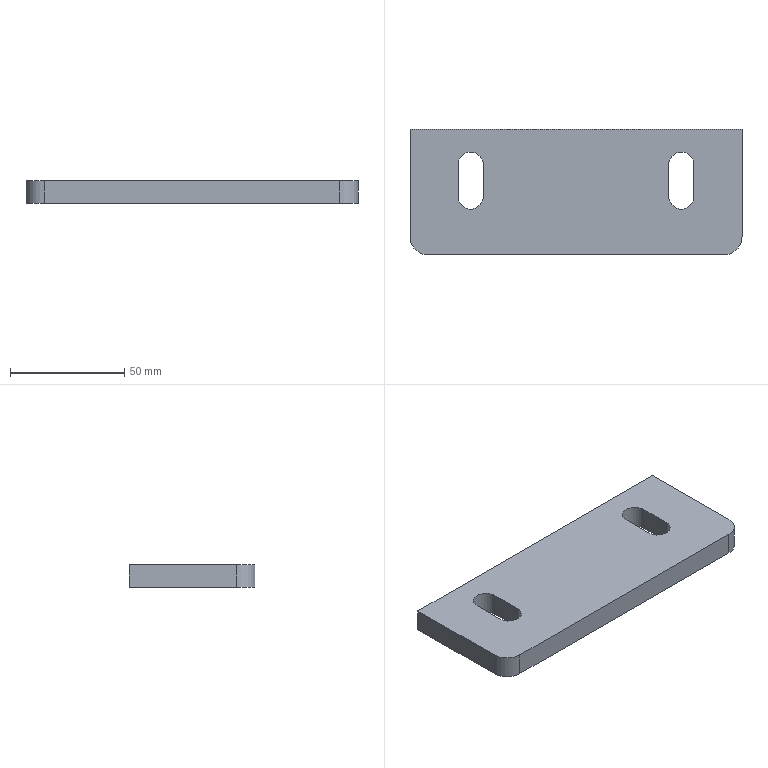Part | SolidWorks | features Extrusion 1, Fillet 1, ICE 1 | 1 solid | 16 faces | box 145 x 55 x 10 mm | volume 74495 mm3 | plane 10 | cylinder 6 | commonest cylinder face diameters 11 x4 16 x2
STEP:
#1=CARTESIAN_POINT('',(-72.5,27.5,0.));
#2=VERTEX_POINT('',#1);
#3=CARTESIAN_POINT('',(-72.5,-19.5,0.));
#4=VERTEX_POINT('',#3);
#5=CARTESIAN_POINT('',(-72.5,27.5,0.));
#6=DIRECTION('',(0.,-1.,0.));
#7=VECTOR('',#6,1000.);
#8=LINE('',#5,#7);
#9=EDGE_CURVE('',#2,#4,#8,.T.);
#10=ORIENTED_EDGE('',*,*,#9,.T.);
#11=CARTESIAN_POINT('',(-72.5,-19.5,10.));
#12=VERTEX_POINT('',#11);
#13=CARTESIAN_POINT('',(-72.5,-19.5,10.));
#14=DIRECTION('',(0.,0.,1.));
#15=VECTOR('',#14,1000.);
#16=LINE('',#13,#15);
#17=EDGE_CURVE('',#4,#12,#16,.T.);
#18=ORIENTED_EDGE('',*,*,#17,.T.);
#19=CARTESIAN_POINT('',(-72.5,27.5,10.));
#20=VERTEX_POINT('',#19);
#21=CARTESIAN_POINT('',(-72.5,27.5,10.));
#22=DIRECTION('',(0.,-1.,0.));
#23=VECTOR('',#22,1000.);
#24=LINE('',#21,#23);
#25=EDGE_CURVE('',#20,#12,#24,.T.);
#26=ORIENTED_EDGE('',*,*,#25,.F.);
#27=CARTESIAN_POINT('',(-72.5,27.5,10.));
#28=DIRECTION('',(0.,0.,-1.));
#29=VECTOR('',#28,1000.);
#30=LINE('',#27,#29);
#31=EDGE_CURVE('',#20,#2,#30,.T.);
#32=ORIENTED_EDGE('',*,*,#31,.T.);
#33=EDGE_LOOP('',(#10,#18,#26,#32));
#34=FACE_OUTER_BOUND('',#33,.T.);
#35=CARTESIAN_POINT('',(-72.5,27.5,10.));
#36=DIRECTION('',(1.,0.,0.));
#37=DIRECTION('',(0.,1.,0.));
#38=AXIS2_PLACEMENT_3D('',#35,#36,#37);
#39=PLANE('',#38);
#40=ADVANCED_FACE('',(#34),#39,.F.);
#41=CARTESIAN_POINT('',(-64.5,-27.5,0.));
#42=VERTEX_POINT('',#41);
#43=CARTESIAN_POINT('',(64.5,-27.5,0.));
#44=VERTEX_POINT('',#43);
#45=CARTESIAN_POINT('',(72.5,-27.5,0.));
#46=DIRECTION('',(1.,0.,0.));
#47=VECTOR('',#46,1000.);
#48=LINE('',#45,#47);
#49=EDGE_CURVE('',#42,#44,#48,.T.);
#50=ORIENTED_EDGE('',*,*,#49,.T.);
#51=CARTESIAN_POINT('',(64.5,-27.5,10.));
#52=VERTEX_POINT('',#51);
#53=CARTESIAN_POINT('',(64.5,-27.5,10.));
#54=DIRECTION('',(0.,0.,1.));
#55=VECTOR('',#54,1000.);
#56=LINE('',#53,#55);
#57=EDGE_CURVE('',#44,#52,#56,.T.);
#58=ORIENTED_EDGE('',*,*,#57,.T.);
#59=CARTESIAN_POINT('',(-64.5,-27.5,10.));
#60=VERTEX_POINT('',#59);
#61=CARTESIAN_POINT('',(72.5,-27.5,10.));
#62=DIRECTION('',(1.,0.,0.));
#63=VECTOR('',#62,1000.);
#64=LINE('',#61,#63);
#65=EDGE_CURVE('',#60,#52,#64,.T.);
#66=ORIENTED_EDGE('',*,*,#65,.F.);
#67=CARTESIAN_POINT('',(-64.5,-27.5,10.));
#68=DIRECTION('',(0.,0.,-1.));
#69=VECTOR('',#68,1000.);
#70=LINE('',#67,#69);
#71=EDGE_CURVE('',#60,#42,#70,.T.);
#72=ORIENTED_EDGE('',*,*,#71,.T.);
#73=EDGE_LOOP('',(#50,#58,#66,#72));
#74=FACE_OUTER_BOUND('',#73,.T.);
#75=CARTESIAN_POINT('',(72.5,-27.5,10.));
#76=DIRECTION('',(0.,1.,0.));
#77=DIRECTION('',(-1.,0.,0.));
#78=AXIS2_PLACEMENT_3D('',#75,#76,#77);
#79=PLANE('',#78);
#80=ADVANCED_FACE('',(#74),#79,.F.);
#81=CARTESIAN_POINT('',(72.5,-19.5,10.));
#82=VERTEX_POINT('',#81);
#83=CARTESIAN_POINT('',(72.5,27.5,10.));
#84=VERTEX_POINT('',#83);
#85=CARTESIAN_POINT('',(72.5,27.5,10.));
#86=DIRECTION('',(0.,1.,0.));
#87=VECTOR('',#86,1000.);
#88=LINE('',#85,#87);
#89=EDGE_CURVE('',#82,#84,#88,.T.);
#90=ORIENTED_EDGE('',*,*,#89,.F.);
#91=CARTESIAN_POINT('',(72.5,-19.5,0.));
#92=VERTEX_POINT('',#91);
#93=CARTESIAN_POINT('',(72.5,-19.5,10.));
#94=DIRECTION('',(0.,0.,-1.));
#95=VECTOR('',#94,1000.);
#96=LINE('',#93,#95);
#97=EDGE_CURVE('',#82,#92,#96,.T.);
#98=ORIENTED_EDGE('',*,*,#97,.T.);
#99=CARTESIAN_POINT('',(72.5,27.5,0.));
#100=VERTEX_POINT('',#99);
#101=CARTESIAN_POINT('',(72.5,27.5,0.));
#102=DIRECTION('',(0.,1.,0.));
#103=VECTOR('',#102,1000.);
#104=LINE('',#101,#103);
#105=EDGE_CURVE('',#92,#100,#104,.T.);
#106=ORIENTED_EDGE('',*,*,#105,.T.);
#107=CARTESIAN_POINT('',(72.5,27.5,10.));
#108=DIRECTION('',(0.,0.,-1.));
#109=VECTOR('',#108,1000.);
#110=LINE('',#107,#109);
#111=EDGE_CURVE('',#84,#100,#110,.T.);
#112=ORIENTED_EDGE('',*,*,#111,.F.);
#113=EDGE_LOOP('',(#90,#98,#106,#112));
#114=FACE_OUTER_BOUND('',#113,.T.);
#115=CARTESIAN_POINT('',(72.5,27.5,10.));
#116=DIRECTION('',(-1.,0.,0.));
#117=DIRECTION('',(0.,0.,1.));
#118=AXIS2_PLACEMENT_3D('',#115,#116,#117);
#119=PLANE('',#118);
#120=ADVANCED_FACE('',(#114),#119,.F.);
#121=CARTESIAN_POINT('',(72.5,27.5,0.));
#122=DIRECTION('',(-1.,0.,0.));
#123=VECTOR('',#122,1000.);
#124=LINE('',#121,#123);
#125=EDGE_CURVE('',#100,#2,#124,.T.);
#126=ORIENTED_EDGE('',*,*,#125,.T.);
#127=ORIENTED_EDGE('',*,*,#31,.F.);
#128=CARTESIAN_POINT('',(72.5,27.5,10.));
#129=DIRECTION('',(-1.,0.,0.));
#130=VECTOR('',#129,1000.);
#131=LINE('',#128,#130);
#132=EDGE_CURVE('',#84,#20,#131,.T.);
#133=ORIENTED_EDGE('',*,*,#132,.F.);
#134=ORIENTED_EDGE('',*,*,#111,.T.);
#135=EDGE_LOOP('',(#126,#127,#133,#134));
#136=FACE_OUTER_BOUND('',#135,.T.);
#137=CARTESIAN_POINT('',(72.5,27.5,10.));
#138=DIRECTION('',(0.,-1.,0.));
#139=DIRECTION('',(1.,0.,0.));
#140=AXIS2_PLACEMENT_3D('',#137,#138,#139);
#141=PLANE('',#140);
#142=ADVANCED_FACE('',(#136),#141,.F.);
#143=CARTESIAN_POINT('',(40.5,12.,10.));
#144=VERTEX_POINT('',#143);
#145=CARTESIAN_POINT('',(40.5,-2.,10.));
#146=VERTEX_POINT('',#145);
#147=CARTESIAN_POINT('',(40.5,12.,10.));
#148=DIRECTION('',(0.,-1.,0.));
#149=VECTOR('',#148,1000.);
#150=LINE('',#147,#149);
#151=EDGE_CURVE('',#144,#146,#150,.T.);
#152=ORIENTED_EDGE('',*,*,#151,.F.);
#153=CARTESIAN_POINT('',(51.5,12.,10.));
#154=VERTEX_POINT('',#153);
#155=CARTESIAN_POINT('',(46.,12.,10.));
#156=DIRECTION('',(0.,0.,1.));
#157=DIRECTION('',(1.,0.,0.));
#158=AXIS2_PLACEMENT_3D('',#155,#156,#157);
#159=CIRCLE('',#158,5.5);
#160=EDGE_CURVE('',#154,#144,#159,.T.);
#161=ORIENTED_EDGE('',*,*,#160,.F.);
#162=CARTESIAN_POINT('',(51.5,-2.,10.));
#163=VERTEX_POINT('',#162);
#164=CARTESIAN_POINT('',(51.5,12.,10.));
#165=DIRECTION('',(0.,1.,0.));
#166=VECTOR('',#165,1000.);
#167=LINE('',#164,#166);
#168=EDGE_CURVE('',#163,#154,#167,.T.);
#169=ORIENTED_EDGE('',*,*,#168,.F.);
#170=CARTESIAN_POINT('',(46.,-2.,10.));
#171=DIRECTION('',(0.,0.,1.));
#172=DIRECTION('',(1.,0.,0.));
#173=AXIS2_PLACEMENT_3D('',#170,#171,#172);
#174=CIRCLE('',#173,5.5);
#175=EDGE_CURVE('',#146,#163,#174,.T.);
#176=ORIENTED_EDGE('',*,*,#175,.F.);
#177=EDGE_LOOP('',(#152,#161,#169,#176));
#178=FACE_BOUND('',#177,.T.);
#179=CARTESIAN_POINT('',(-51.5,12.,10.));
#180=VERTEX_POINT('',#179);
#181=CARTESIAN_POINT('',(-51.5,-2.,10.));
#182=VERTEX_POINT('',#181);
#183=CARTESIAN_POINT('',(-51.5,12.,10.));
#184=DIRECTION('',(0.,-1.,0.));
#185=VECTOR('',#184,1000.);
#186=LINE('',#183,#185);
#187=EDGE_CURVE('',#180,#182,#186,.T.);
#188=ORIENTED_EDGE('',*,*,#187,.F.);
#189=CARTESIAN_POINT('',(-40.5,12.,10.));
#190=VERTEX_POINT('',#189);
#191=CARTESIAN_POINT('',(-46.,12.,10.));
#192=DIRECTION('',(0.,0.,1.));
#193=DIRECTION('',(1.,0.,0.));
#194=AXIS2_PLACEMENT_3D('',#191,#192,#193);
#195=CIRCLE('',#194,5.5);
#196=EDGE_CURVE('',#190,#180,#195,.T.);
#197=ORIENTED_EDGE('',*,*,#196,.F.);
#198=CARTESIAN_POINT('',(-40.5,-2.,10.));
#199=VERTEX_POINT('',#198);
#200=CARTESIAN_POINT('',(-40.5,12.,10.));
#201=DIRECTION('',(0.,1.,0.));
#202=VECTOR('',#201,1000.);
#203=LINE('',#200,#202);
#204=EDGE_CURVE('',#199,#190,#203,.T.);
#205=ORIENTED_EDGE('',*,*,#204,.F.);
#206=CARTESIAN_POINT('',(-46.,-2.,10.));
#207=DIRECTION('',(0.,0.,1.));
#208=DIRECTION('',(1.,0.,0.));
#209=AXIS2_PLACEMENT_3D('',#206,#207,#208);
#210=CIRCLE('',#209,5.5);
#211=EDGE_CURVE('',#182,#199,#210,.T.);
#212=ORIENTED_EDGE('',*,*,#211,.F.);
#213=EDGE_LOOP('',(#188,#197,#205,#212));
#214=FACE_BOUND('',#213,.T.);
#215=ORIENTED_EDGE('',*,*,#65,.T.);
#216=CARTESIAN_POINT('',(64.5,-19.5,10.));
#217=DIRECTION('',(0.,0.,1.));
#218=DIRECTION('',(-1.,0.,0.));
#219=AXIS2_PLACEMENT_3D('',#216,#217,#218);
#220=CIRCLE('',#219,8.);
#221=EDGE_CURVE('',#52,#82,#220,.T.);
#222=ORIENTED_EDGE('',*,*,#221,.T.);
#223=ORIENTED_EDGE('',*,*,#89,.T.);
#224=ORIENTED_EDGE('',*,*,#132,.T.);
#225=ORIENTED_EDGE('',*,*,#25,.T.);
#226=CARTESIAN_POINT('',(-64.5,-19.5,10.));
#227=DIRECTION('',(0.,0.,1.));
#228=DIRECTION('',(-1.,0.,0.));
#229=AXIS2_PLACEMENT_3D('',#226,#227,#228);
#230=CIRCLE('',#229,8.);
#231=EDGE_CURVE('',#12,#60,#230,.T.);
#232=ORIENTED_EDGE('',*,*,#231,.T.);
#233=EDGE_LOOP('',(#215,#222,#223,#224,#225,#232));
#234=FACE_OUTER_BOUND('',#233,.T.);
#235=CARTESIAN_POINT('',(0.,0.,10.));
#236=DIRECTION('',(0.,0.,-1.));
#237=DIRECTION('',(-1.,0.,0.));
#238=AXIS2_PLACEMENT_3D('',#235,#236,#237);
#239=PLANE('',#238);
#240=ADVANCED_FACE('',(#178,#214,#234),#239,.F.);
#241=CARTESIAN_POINT('',(51.5,12.,0.));
#242=VERTEX_POINT('',#241);
#243=CARTESIAN_POINT('',(40.5,12.,0.));
#244=VERTEX_POINT('',#243);
#245=CARTESIAN_POINT('',(46.,12.,0.));
#246=DIRECTION('',(0.,0.,1.));
#247=DIRECTION('',(1.,0.,0.));
#248=AXIS2_PLACEMENT_3D('',#245,#246,#247);
#249=CIRCLE('',#248,5.5);
#250=EDGE_CURVE('',#242,#244,#249,.T.);
#251=ORIENTED_EDGE('',*,*,#250,.T.);
#252=CARTESIAN_POINT('',(40.5,-2.,0.));
#253=VERTEX_POINT('',#252);
#254=CARTESIAN_POINT('',(40.5,12.,0.));
#255=DIRECTION('',(0.,-1.,0.));
#256=VECTOR('',#255,1000.);
#257=LINE('',#254,#256);
#258=EDGE_CURVE('',#244,#253,#257,.T.);
#259=ORIENTED_EDGE('',*,*,#258,.T.);
#260=CARTESIAN_POINT('',(51.5,-2.,0.));
#261=VERTEX_POINT('',#260);
#262=CARTESIAN_POINT('',(46.,-2.,0.));
#263=DIRECTION('',(0.,0.,1.));
#264=DIRECTION('',(1.,0.,0.));
#265=AXIS2_PLACEMENT_3D('',#262,#263,#264);
#266=CIRCLE('',#265,5.5);
#267=EDGE_CURVE('',#253,#261,#266,.T.);
#268=ORIENTED_EDGE('',*,*,#267,.T.);
#269=CARTESIAN_POINT('',(51.5,12.,0.));
#270=DIRECTION('',(0.,1.,0.));
#271=VECTOR('',#270,1000.);
#272=LINE('',#269,#271);
#273=EDGE_CURVE('',#261,#242,#272,.T.);
#274=ORIENTED_EDGE('',*,*,#273,.T.);
#275=EDGE_LOOP('',(#251,#259,#268,#274));
#276=FACE_BOUND('',#275,.T.);
#277=CARTESIAN_POINT('',(-40.5,12.,0.));
#278=VERTEX_POINT('',#277);
#279=CARTESIAN_POINT('',(-51.5,12.,0.));
#280=VERTEX_POINT('',#279);
#281=CARTESIAN_POINT('',(-46.,12.,0.));
#282=DIRECTION('',(0.,0.,1.));
#283=DIRECTION('',(1.,0.,0.));
#284=AXIS2_PLACEMENT_3D('',#281,#282,#283);
#285=CIRCLE('',#284,5.5);
#286=EDGE_CURVE('',#278,#280,#285,.T.);
#287=ORIENTED_EDGE('',*,*,#286,.T.);
#288=CARTESIAN_POINT('',(-51.5,-2.,0.));
#289=VERTEX_POINT('',#288);
#290=CARTESIAN_POINT('',(-51.5,12.,0.));
#291=DIRECTION('',(0.,-1.,0.));
#292=VECTOR('',#291,1000.);
#293=LINE('',#290,#292);
#294=EDGE_CURVE('',#280,#289,#293,.T.);
#295=ORIENTED_EDGE('',*,*,#294,.T.);
#296=CARTESIAN_POINT('',(-40.5,-2.,0.));
#297=VERTEX_POINT('',#296);
#298=CARTESIAN_POINT('',(-46.,-2.,0.));
#299=DIRECTION('',(0.,0.,1.));
#300=DIRECTION('',(1.,0.,0.));
#301=AXIS2_PLACEMENT_3D('',#298,#299,#300);
#302=CIRCLE('',#301,5.5);
#303=EDGE_CURVE('',#289,#297,#302,.T.);
#304=ORIENTED_EDGE('',*,*,#303,.T.);
#305=CARTESIAN_POINT('',(-40.5,12.,0.));
#306=DIRECTION('',(0.,1.,0.));
#307=VECTOR('',#306,1000.);
#308=LINE('',#305,#307);
#309=EDGE_CURVE('',#297,#278,#308,.T.);
#310=ORIENTED_EDGE('',*,*,#309,.T.);
#311=EDGE_LOOP('',(#287,#295,#304,#310));
#312=FACE_BOUND('',#311,.T.);
#313=ORIENTED_EDGE('',*,*,#105,.F.);
#314=CARTESIAN_POINT('',(64.5,-19.5,0.));
#315=DIRECTION('',(0.,0.,-1.));
#316=DIRECTION('',(-1.,0.,0.));
#317=AXIS2_PLACEMENT_3D('',#314,#315,#316);
#318=CIRCLE('',#317,8.);
#319=EDGE_CURVE('',#92,#44,#318,.T.);
#320=ORIENTED_EDGE('',*,*,#319,.T.);
#321=ORIENTED_EDGE('',*,*,#49,.F.);
#322=CARTESIAN_POINT('',(-64.5,-19.5,0.));
#323=DIRECTION('',(0.,0.,-1.));
#324=DIRECTION('',(-1.,0.,0.));
#325=AXIS2_PLACEMENT_3D('',#322,#323,#324);
#326=CIRCLE('',#325,8.);
#327=EDGE_CURVE('',#42,#4,#326,.T.);
#328=ORIENTED_EDGE('',*,*,#327,.T.);
#329=ORIENTED_EDGE('',*,*,#9,.F.);
#330=ORIENTED_EDGE('',*,*,#125,.F.);
#331=EDGE_LOOP('',(#313,#320,#321,#328,#329,#330));
#332=FACE_OUTER_BOUND('',#331,.T.);
#333=CARTESIAN_POINT('',(0.,0.,0.));
#334=DIRECTION('',(0.,0.,-1.));
#335=DIRECTION('',(-1.,0.,0.));
#336=AXIS2_PLACEMENT_3D('',#333,#334,#335);
#337=PLANE('',#336);
#338=ADVANCED_FACE('',(#276,#312,#332),#337,.T.);
#339=ORIENTED_EDGE('',*,*,#221,.F.);
#340=ORIENTED_EDGE('',*,*,#57,.F.);
#341=ORIENTED_EDGE('',*,*,#319,.F.);
#342=ORIENTED_EDGE('',*,*,#97,.F.);
#343=EDGE_LOOP('',(#339,#340,#341,#342));
#344=FACE_OUTER_BOUND('',#343,.T.);
#345=CARTESIAN_POINT('',(64.5,-19.5,10.));
#346=DIRECTION('',(0.,0.,-1.));
#347=DIRECTION('',(-1.,0.,0.));
#348=AXIS2_PLACEMENT_3D('',#345,#346,#347);
#349=CYLINDRICAL_SURFACE('',#348,8.);
#350=ADVANCED_FACE('',(#344),#349,.T.);
#351=ORIENTED_EDGE('',*,*,#231,.F.);
#352=ORIENTED_EDGE('',*,*,#17,.F.);
#353=ORIENTED_EDGE('',*,*,#327,.F.);
#354=ORIENTED_EDGE('',*,*,#71,.F.);
#355=EDGE_LOOP('',(#351,#352,#353,#354));
#356=FACE_OUTER_BOUND('',#355,.T.);
#357=CARTESIAN_POINT('',(-64.5,-19.5,10.));
#358=DIRECTION('',(0.,0.,-1.));
#359=DIRECTION('',(-1.,0.,0.));
#360=AXIS2_PLACEMENT_3D('',#357,#358,#359);
#361=CYLINDRICAL_SURFACE('',#360,8.);
#362=ADVANCED_FACE('',(#356),#361,.T.);
#363=ORIENTED_EDGE('',*,*,#196,.T.);
#364=CARTESIAN_POINT('',(-51.5,12.,0.));
#365=DIRECTION('',(0.,0.,1.));
#366=VECTOR('',#365,1000.);
#367=LINE('',#364,#366);
#368=EDGE_CURVE('',#280,#180,#367,.T.);
#369=ORIENTED_EDGE('',*,*,#368,.F.);
#370=ORIENTED_EDGE('',*,*,#286,.F.);
#371=CARTESIAN_POINT('',(-40.5,12.,0.));
#372=DIRECTION('',(0.,0.,1.));
#373=VECTOR('',#372,1000.);
#374=LINE('',#371,#373);
#375=EDGE_CURVE('',#278,#190,#374,.T.);
#376=ORIENTED_EDGE('',*,*,#375,.T.);
#377=EDGE_LOOP('',(#363,#369,#370,#376));
#378=FACE_OUTER_BOUND('',#377,.T.);
#379=CARTESIAN_POINT('',(-46.,12.,0.));
#380=DIRECTION('',(0.,0.,1.));
#381=DIRECTION('',(1.,0.,0.));
#382=AXIS2_PLACEMENT_3D('',#379,#380,#381);
#383=CYLINDRICAL_SURFACE('',#382,5.5);
#384=ADVANCED_FACE('',(#378),#383,.F.);
#385=ORIENTED_EDGE('',*,*,#204,.T.);
#386=ORIENTED_EDGE('',*,*,#375,.F.);
#387=ORIENTED_EDGE('',*,*,#309,.F.);
#388=CARTESIAN_POINT('',(-40.5,-2.,0.));
#389=DIRECTION('',(0.,0.,1.));
#390=VECTOR('',#389,1000.);
#391=LINE('',#388,#390);
#392=EDGE_CURVE('',#297,#199,#391,.T.);
#393=ORIENTED_EDGE('',*,*,#392,.T.);
#394=EDGE_LOOP('',(#385,#386,#387,#393));
#395=FACE_OUTER_BOUND('',#394,.T.);
#396=CARTESIAN_POINT('',(-40.5,12.,0.));
#397=DIRECTION('',(1.,0.,0.));
#398=DIRECTION('',(0.,0.,-1.));
#399=AXIS2_PLACEMENT_3D('',#396,#397,#398);
#400=PLANE('',#399);
#401=ADVANCED_FACE('',(#395),#400,.F.);
#402=ORIENTED_EDGE('',*,*,#211,.T.);
#403=ORIENTED_EDGE('',*,*,#392,.F.);
#404=ORIENTED_EDGE('',*,*,#303,.F.);
#405=CARTESIAN_POINT('',(-51.5,-2.,0.));
#406=DIRECTION('',(0.,0.,1.));
#407=VECTOR('',#406,1000.);
#408=LINE('',#405,#407);
#409=EDGE_CURVE('',#289,#182,#408,.T.);
#410=ORIENTED_EDGE('',*,*,#409,.T.);
#411=EDGE_LOOP('',(#402,#403,#404,#410));
#412=FACE_OUTER_BOUND('',#411,.T.);
#413=CARTESIAN_POINT('',(-46.,-2.,0.));
#414=DIRECTION('',(0.,0.,1.));
#415=DIRECTION('',(1.,0.,0.));
#416=AXIS2_PLACEMENT_3D('',#413,#414,#415);
#417=CYLINDRICAL_SURFACE('',#416,5.5);
#418=ADVANCED_FACE('',(#412),#417,.F.);
#419=ORIENTED_EDGE('',*,*,#187,.T.);
#420=ORIENTED_EDGE('',*,*,#409,.F.);
#421=ORIENTED_EDGE('',*,*,#294,.F.);
#422=ORIENTED_EDGE('',*,*,#368,.T.);
#423=EDGE_LOOP('',(#419,#420,#421,#422));
#424=FACE_OUTER_BOUND('',#423,.T.);
#425=CARTESIAN_POINT('',(-51.5,12.,0.));
#426=DIRECTION('',(-1.,0.,0.));
#427=DIRECTION('',(0.,0.,1.));
#428=AXIS2_PLACEMENT_3D('',#425,#426,#427);
#429=PLANE('',#428);
#430=ADVANCED_FACE('',(#424),#429,.F.);
#431=ORIENTED_EDGE('',*,*,#160,.T.);
#432=CARTESIAN_POINT('',(40.5,12.,0.));
#433=DIRECTION('',(0.,0.,1.));
#434=VECTOR('',#433,1000.);
#435=LINE('',#432,#434);
#436=EDGE_CURVE('',#244,#144,#435,.T.);
#437=ORIENTED_EDGE('',*,*,#436,.F.);
#438=ORIENTED_EDGE('',*,*,#250,.F.);
#439=CARTESIAN_POINT('',(51.5,12.,0.));
#440=DIRECTION('',(0.,0.,1.));
#441=VECTOR('',#440,1000.);
#442=LINE('',#439,#441);
#443=EDGE_CURVE('',#242,#154,#442,.T.);
#444=ORIENTED_EDGE('',*,*,#443,.T.);
#445=EDGE_LOOP('',(#431,#437,#438,#444));
#446=FACE_OUTER_BOUND('',#445,.T.);
#447=CARTESIAN_POINT('',(46.,12.,0.));
#448=DIRECTION('',(0.,0.,1.));
#449=DIRECTION('',(1.,0.,0.));
#450=AXIS2_PLACEMENT_3D('',#447,#448,#449);
#451=CYLINDRICAL_SURFACE('',#450,5.5);
#452=ADVANCED_FACE('',(#446),#451,.F.);
#453=ORIENTED_EDGE('',*,*,#168,.T.);
#454=ORIENTED_EDGE('',*,*,#443,.F.);
#455=ORIENTED_EDGE('',*,*,#273,.F.);
#456=CARTESIAN_POINT('',(51.5,-2.,0.));
#457=DIRECTION('',(0.,0.,1.));
#458=VECTOR('',#457,1000.);
#459=LINE('',#456,#458);
#460=EDGE_CURVE('',#261,#163,#459,.T.);
#461=ORIENTED_EDGE('',*,*,#460,.T.);
#462=EDGE_LOOP('',(#453,#454,#455,#461));
#463=FACE_OUTER_BOUND('',#462,.T.);
#464=CARTESIAN_POINT('',(51.5,12.,0.));
#465=DIRECTION('',(1.,0.,0.));
#466=DIRECTION('',(0.,0.,-1.));
#467=AXIS2_PLACEMENT_3D('',#464,#465,#466);
#468=PLANE('',#467);
#469=ADVANCED_FACE('',(#463),#468,.F.);
#470=ORIENTED_EDGE('',*,*,#175,.T.);
#471=ORIENTED_EDGE('',*,*,#460,.F.);
#472=ORIENTED_EDGE('',*,*,#267,.F.);
#473=CARTESIAN_POINT('',(40.5,-2.,0.));
#474=DIRECTION('',(0.,0.,1.));
#475=VECTOR('',#474,1000.);
#476=LINE('',#473,#475);
#477=EDGE_CURVE('',#253,#146,#476,.T.);
#478=ORIENTED_EDGE('',*,*,#477,.T.);
#479=EDGE_LOOP('',(#470,#471,#472,#478));
#480=FACE_OUTER_BOUND('',#479,.T.);
#481=CARTESIAN_POINT('',(46.,-2.,0.));
#482=DIRECTION('',(0.,0.,1.));
#483=DIRECTION('',(1.,0.,0.));
#484=AXIS2_PLACEMENT_3D('',#481,#482,#483);
#485=CYLINDRICAL_SURFACE('',#484,5.5);
#486=ADVANCED_FACE('',(#480),#485,.F.);
#487=ORIENTED_EDGE('',*,*,#151,.T.);
#488=ORIENTED_EDGE('',*,*,#477,.F.);
#489=ORIENTED_EDGE('',*,*,#258,.F.);
#490=ORIENTED_EDGE('',*,*,#436,.T.);
#491=EDGE_LOOP('',(#487,#488,#489,#490));
#492=FACE_OUTER_BOUND('',#491,.T.);
#493=CARTESIAN_POINT('',(40.5,12.,0.));
#494=DIRECTION('',(-1.,0.,0.));
#495=DIRECTION('',(0.,0.,1.));
#496=AXIS2_PLACEMENT_3D('',#493,#494,#495);
#497=PLANE('',#496);
#498=ADVANCED_FACE('',(#492),#497,.F.);
#499=CLOSED_SHELL('',(#40,#80,#120,#142,#240,#338,#350,#362,#384,#401,#418,#430,#452,#469,#486,#498));
#500=MANIFOLD_SOLID_BREP('',#499);
#501=CARTESIAN_POINT('',(0.,0.,0.));
#502=DIRECTION('',(0.,0.,1.));
#503=DIRECTION('',(1.,0.,0.));
#504=AXIS2_PLACEMENT_3D('',#501,#502,#503);
#505=(LENGTH_UNIT()NAMED_UNIT(*)SI_UNIT(.MILLI.,.METRE.));
#506=UNCERTAINTY_MEASURE_WITH_UNIT(LENGTH_MEASURE(0.00001),#505,'','');
#507=(NAMED_UNIT(*)PLANE_ANGLE_UNIT()SI_UNIT($,.RADIAN.));
#508=(NAMED_UNIT(*)SI_UNIT($,.STERADIAN.)SOLID_ANGLE_UNIT());
#509=(GEOMETRIC_REPRESENTATION_CONTEXT(3)GLOBAL_UNCERTAINTY_ASSIGNED_CONTEXT((#506))GLOBAL_UNIT_ASSIGNED_CONTEXT((#505,#507,#508))REPRESENTATION_CONTEXT('',''));
#510=ADVANCED_BREP_SHAPE_REPRESENTATION('',(#500,#504),#509);